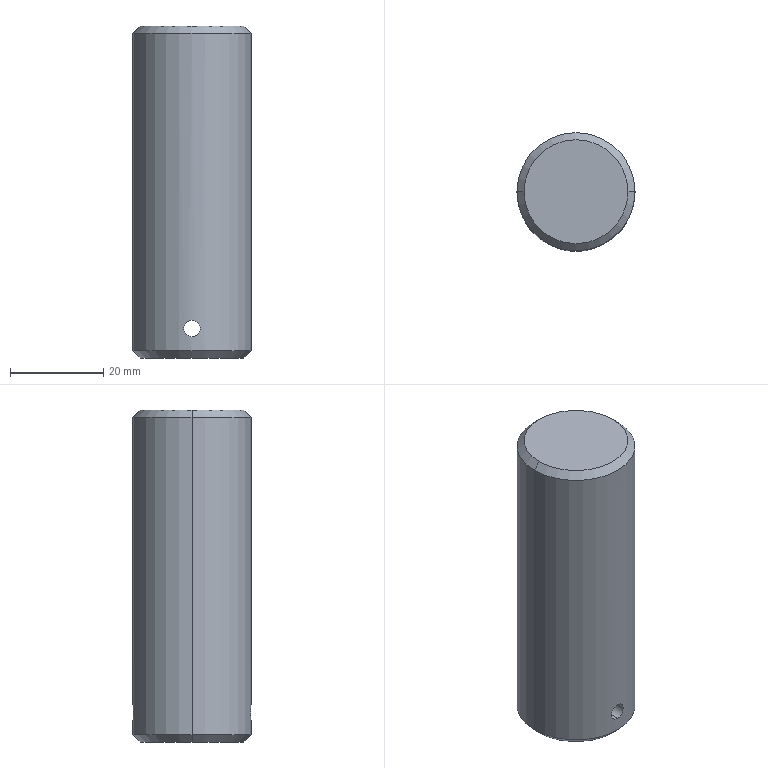Part | SolidWorks | features Chamfer 1, Extrusion 1, ICE 1 | 1 solid | 10 faces | box 25.4 x 25.4 x 71.37 mm | volume 35732 mm3 | cylinder 4 | cone 4 | plane 2 | commonest cylinder face diameters 3.57 x2 25.4 x2
STEP:
#1=CARTESIAN_POINT('',(0.,-12.7,4.565));
#2=VERTEX_POINT('',#1);
#3=CARTESIAN_POINT('',(0.,-12.7,8.135));
#4=VERTEX_POINT('',#3);
#5=CARTESIAN_POINT('',(0.,-12.7,4.565));
#6=CARTESIAN_POINT('',(-0.2331,-12.7,4.565));
#7=CARTESIAN_POINT('',(-0.4682,-12.693,4.612));
#8=CARTESIAN_POINT('',(-0.8979,-12.67,4.79));
#9=CARTESIAN_POINT('',(-1.097,-12.654,4.923));
#10=CARTESIAN_POINT('',(-1.344,-12.629,5.169));
#11=CARTESIAN_POINT('',(-1.419,-12.621,5.261));
#12=CARTESIAN_POINT('',(-1.549,-12.605,5.455));
#13=CARTESIAN_POINT('',(-1.603,-12.598,5.557));
#14=CARTESIAN_POINT('',(-1.693,-12.587,5.773));
#15=CARTESIAN_POINT('',(-1.728,-12.582,5.886));
#16=CARTESIAN_POINT('',(-1.773,-12.576,6.115));
#17=CARTESIAN_POINT('',(-1.785,-12.574,6.231));
#18=CARTESIAN_POINT('',(-1.785,-12.574,6.467));
#19=CARTESIAN_POINT('',(-1.774,-12.576,6.583));
#20=CARTESIAN_POINT('',(-1.728,-12.582,6.811));
#21=CARTESIAN_POINT('',(-1.694,-12.587,6.925));
#22=CARTESIAN_POINT('',(-1.605,-12.598,7.141));
#23=CARTESIAN_POINT('',(-1.55,-12.605,7.243));
#24=CARTESIAN_POINT('',(-1.42,-12.62,7.437));
#25=CARTESIAN_POINT('',(-1.345,-12.629,7.529));
#26=CARTESIAN_POINT('',(-1.099,-12.653,7.776));
#27=CARTESIAN_POINT('',(-0.9,-12.67,7.909));
#28=CARTESIAN_POINT('',(-0.4707,-12.693,8.087));
#29=CARTESIAN_POINT('',(-0.2361,-12.7,8.135));
#30=CARTESIAN_POINT('',(0.,-12.7,8.135));
#31=B_SPLINE_CURVE_WITH_KNOTS('',3,(#5,#6,#7,#8,#9,#10,#11,#12,#13,#14,#15,#16,#17,#18,#19,#20,#21,#22,#23,#24,#25,#26,#27,#28,#29,#30),.UNSPECIFIED.,.F.,.F.,(4,2,2,2,2,2,2,2,2,2,2,2,4),(0.005588,0.006286,0.006984,0.007333,0.007682,0.008032,0.008381,0.00873,0.009079,0.009428,0.009777,0.01048,0.01117),.UNSPECIFIED.);
#32=EDGE_CURVE('',#2,#4,#31,.T.);
#33=ORIENTED_EDGE('',*,*,#32,.F.);
#34=CARTESIAN_POINT('',(0.,12.7,4.565));
#35=VERTEX_POINT('',#34);
#36=CARTESIAN_POINT('',(0.,-12.7,4.565));
#37=DIRECTION('',(0.,1.,0.));
#38=VECTOR('',#37,1000.);
#39=LINE('',#36,#38);
#40=EDGE_CURVE('',#2,#35,#39,.T.);
#41=ORIENTED_EDGE('',*,*,#40,.T.);
#42=CARTESIAN_POINT('',(0.,12.7,8.135));
#43=VERTEX_POINT('',#42);
#44=CARTESIAN_POINT('',(0.,12.7,8.135));
#45=CARTESIAN_POINT('',(-0.1181,12.7,8.135));
#46=CARTESIAN_POINT('',(-0.2342,12.698,8.123));
#47=CARTESIAN_POINT('',(-0.4625,12.692,8.078));
#48=CARTESIAN_POINT('',(-0.576,12.687,8.044));
#49=CARTESIAN_POINT('',(-0.7921,12.676,7.954));
#50=CARTESIAN_POINT('',(-0.8946,12.669,7.899));
#51=CARTESIAN_POINT('',(-1.089,12.654,7.769));
#52=CARTESIAN_POINT('',(-1.18,12.645,7.694));
#53=CARTESIAN_POINT('',(-1.427,12.621,7.447));
#54=CARTESIAN_POINT('',(-1.56,12.604,7.248));
#55=CARTESIAN_POINT('',(-1.738,12.581,6.819));
#56=CARTESIAN_POINT('',(-1.785,12.574,6.584));
#57=CARTESIAN_POINT('',(-1.785,12.574,6.234));
#58=CARTESIAN_POINT('',(-1.773,12.576,6.116));
#59=CARTESIAN_POINT('',(-1.728,12.582,5.887));
#60=CARTESIAN_POINT('',(-1.694,12.587,5.775));
#61=CARTESIAN_POINT('',(-1.604,12.598,5.559));
#62=CARTESIAN_POINT('',(-1.549,12.605,5.455));
#63=CARTESIAN_POINT('',(-1.419,12.621,5.261));
#64=CARTESIAN_POINT('',(-1.345,12.629,5.171));
#65=CARTESIAN_POINT('',(-1.179,12.645,5.005));
#66=CARTESIAN_POINT('',(-1.089,12.654,4.931));
#67=CARTESIAN_POINT('',(-0.8958,12.669,4.802));
#68=CARTESIAN_POINT('',(-0.7914,12.676,4.746));
#69=CARTESIAN_POINT('',(-0.5753,12.687,4.656));
#70=CARTESIAN_POINT('',(-0.4641,12.692,4.622));
#71=CARTESIAN_POINT('',(-0.235,12.698,4.577));
#72=CARTESIAN_POINT('',(-0.1166,12.7,4.565));
#73=CARTESIAN_POINT('',(0.,12.7,4.565));
#74=B_SPLINE_CURVE_WITH_KNOTS('',3,(#44,#45,#46,#47,#48,#49,#50,#51,#52,#53,#54,#55,#56,#57,#58,#59,#60,#61,#62,#63,#64,#65,#66,#67,#68,#69,#70,#71,#72,#73),.UNSPECIFIED.,.F.,.F.,(4,2,2,2,2,2,2,2,2,2,2,2,2,2,4),(0.,0.0003492,0.0006985,0.001048,0.001397,0.002095,0.002794,0.003143,0.003492,0.003842,0.004191,0.00454,0.004889,0.005238,0.005588),.UNSPECIFIED.);
#75=EDGE_CURVE('',#43,#35,#74,.T.);
#76=ORIENTED_EDGE('',*,*,#75,.F.);
#77=CARTESIAN_POINT('',(0.,-12.7,8.135));
#78=DIRECTION('',(0.,1.,0.));
#79=VECTOR('',#78,1000.);
#80=LINE('',#77,#79);
#81=EDGE_CURVE('',#4,#43,#80,.T.);
#82=ORIENTED_EDGE('',*,*,#81,.F.);
#83=EDGE_LOOP('',(#33,#41,#76,#82));
#84=FACE_OUTER_BOUND('',#83,.T.);
#85=CARTESIAN_POINT('',(0.,-12.7,6.35));
#86=DIRECTION('',(0.,1.,0.));
#87=DIRECTION('',(0.,0.,1.));
#88=AXIS2_PLACEMENT_3D('',#85,#86,#87);
#89=CYLINDRICAL_SURFACE('',#88,1.785);
#90=ADVANCED_FACE('',(#84),#89,.F.);
#91=CARTESIAN_POINT('',(11.176,0.,71.37));
#92=VERTEX_POINT('',#91);
#93=CARTESIAN_POINT('',(-11.176,0.,71.37));
#94=VERTEX_POINT('',#93);
#95=CARTESIAN_POINT('',(0.,0.,71.37));
#96=DIRECTION('',(0.,0.,1.));
#97=DIRECTION('',(1.,0.,0.));
#98=AXIS2_PLACEMENT_3D('',#95,#96,#97);
#99=CIRCLE('',#98,11.176);
#100=EDGE_CURVE('',#92,#94,#99,.T.);
#101=ORIENTED_EDGE('',*,*,#100,.F.);
#102=CARTESIAN_POINT('',(12.7,0.,69.846));
#103=VERTEX_POINT('',#102);
#104=CARTESIAN_POINT('',(11.176,0.,71.37));
#105=DIRECTION('',(0.7071,0.,-0.7071));
#106=VECTOR('',#105,1000.);
#107=LINE('',#104,#106);
#108=EDGE_CURVE('',#92,#103,#107,.T.);
#109=ORIENTED_EDGE('',*,*,#108,.T.);
#110=CARTESIAN_POINT('',(-12.7,0.,69.846));
#111=VERTEX_POINT('',#110);
#112=CARTESIAN_POINT('',(0.,0.,69.846));
#113=DIRECTION('',(0.,0.,-1.));
#114=DIRECTION('',(1.,0.,0.));
#115=AXIS2_PLACEMENT_3D('',#112,#113,#114);
#116=CIRCLE('',#115,12.7);
#117=EDGE_CURVE('',#111,#103,#116,.T.);
#118=ORIENTED_EDGE('',*,*,#117,.F.);
#119=CARTESIAN_POINT('',(-11.176,0.,71.37));
#120=DIRECTION('',(-0.7071,0.,-0.7071));
#121=VECTOR('',#120,1000.);
#122=LINE('',#119,#121);
#123=EDGE_CURVE('',#94,#111,#122,.T.);
#124=ORIENTED_EDGE('',*,*,#123,.F.);
#125=EDGE_LOOP('',(#101,#109,#118,#124));
#126=FACE_OUTER_BOUND('',#125,.T.);
#127=CARTESIAN_POINT('',(0.,0.,71.37));
#128=DIRECTION('',(0.,0.,-1.));
#129=DIRECTION('',(-1.,0.,0.));
#130=AXIS2_PLACEMENT_3D('',#127,#128,#129);
#131=CONICAL_SURFACE('',#130,11.176,0.7854);
#132=ADVANCED_FACE('',(#126),#131,.T.);
#133=CARTESIAN_POINT('',(-11.176,0.,0.));
#134=VERTEX_POINT('',#133);
#135=CARTESIAN_POINT('',(11.176,0.,0.));
#136=VERTEX_POINT('',#135);
#137=CARTESIAN_POINT('',(0.,0.,0.));
#138=DIRECTION('',(0.,0.,-1.));
#139=DIRECTION('',(1.,0.,0.));
#140=AXIS2_PLACEMENT_3D('',#137,#138,#139);
#141=CIRCLE('',#140,11.176);
#142=EDGE_CURVE('',#134,#136,#141,.T.);
#143=ORIENTED_EDGE('',*,*,#142,.F.);
#144=CARTESIAN_POINT('',(-12.7,0.,1.524));
#145=VERTEX_POINT('',#144);
#146=CARTESIAN_POINT('',(-12.7,0.,1.524));
#147=DIRECTION('',(-0.7071,0.,0.7071));
#148=VECTOR('',#147,1000.);
#149=LINE('',#146,#148);
#150=EDGE_CURVE('',#134,#145,#149,.T.);
#151=ORIENTED_EDGE('',*,*,#150,.T.);
#152=CARTESIAN_POINT('',(12.7,0.,1.524));
#153=VERTEX_POINT('',#152);
#154=CARTESIAN_POINT('',(0.,0.,1.524));
#155=DIRECTION('',(0.,0.,1.));
#156=DIRECTION('',(1.,0.,0.));
#157=AXIS2_PLACEMENT_3D('',#154,#155,#156);
#158=CIRCLE('',#157,12.7);
#159=EDGE_CURVE('',#153,#145,#158,.T.);
#160=ORIENTED_EDGE('',*,*,#159,.F.);
#161=CARTESIAN_POINT('',(12.7,0.,1.524));
#162=DIRECTION('',(0.7071,0.,0.7071));
#163=VECTOR('',#162,1000.);
#164=LINE('',#161,#163);
#165=EDGE_CURVE('',#136,#153,#164,.T.);
#166=ORIENTED_EDGE('',*,*,#165,.F.);
#167=EDGE_LOOP('',(#143,#151,#160,#166));
#168=FACE_OUTER_BOUND('',#167,.T.);
#169=CARTESIAN_POINT('',(0.,0.,1.524));
#170=DIRECTION('',(0.,0.,1.));
#171=DIRECTION('',(1.,0.,0.));
#172=AXIS2_PLACEMENT_3D('',#169,#170,#171);
#173=CONICAL_SURFACE('',#172,12.7,0.7854);
#174=ADVANCED_FACE('',(#168),#173,.T.);
#175=ORIENTED_EDGE('',*,*,#75,.T.);
#176=CARTESIAN_POINT('',(0.,12.7,4.565));
#177=CARTESIAN_POINT('',(0.2331,12.7,4.565));
#178=CARTESIAN_POINT('',(0.4682,12.693,4.612));
#179=CARTESIAN_POINT('',(0.8979,12.67,4.79));
#180=CARTESIAN_POINT('',(1.097,12.654,4.923));
#181=CARTESIAN_POINT('',(1.344,12.629,5.169));
#182=CARTESIAN_POINT('',(1.419,12.621,5.261));
#183=CARTESIAN_POINT('',(1.549,12.605,5.455));
#184=CARTESIAN_POINT('',(1.603,12.598,5.557));
#185=CARTESIAN_POINT('',(1.693,12.587,5.773));
#186=CARTESIAN_POINT('',(1.728,12.582,5.886));
#187=CARTESIAN_POINT('',(1.773,12.576,6.115));
#188=CARTESIAN_POINT('',(1.785,12.574,6.231));
#189=CARTESIAN_POINT('',(1.785,12.574,6.467));
#190=CARTESIAN_POINT('',(1.774,12.576,6.583));
#191=CARTESIAN_POINT('',(1.728,12.582,6.811));
#192=CARTESIAN_POINT('',(1.694,12.587,6.925));
#193=CARTESIAN_POINT('',(1.605,12.598,7.141));
#194=CARTESIAN_POINT('',(1.55,12.605,7.243));
#195=CARTESIAN_POINT('',(1.42,12.62,7.437));
#196=CARTESIAN_POINT('',(1.345,12.629,7.529));
#197=CARTESIAN_POINT('',(1.099,12.653,7.776));
#198=CARTESIAN_POINT('',(0.9,12.67,7.909));
#199=CARTESIAN_POINT('',(0.4707,12.693,8.087));
#200=CARTESIAN_POINT('',(0.2361,12.7,8.135));
#201=CARTESIAN_POINT('',(0.,12.7,8.135));
#202=B_SPLINE_CURVE_WITH_KNOTS('',3,(#176,#177,#178,#179,#180,#181,#182,#183,#184,#185,#186,#187,#188,#189,#190,#191,#192,#193,#194,#195,#196,#197,#198,#199,#200,#201),.UNSPECIFIED.,.F.,.F.,(4,2,2,2,2,2,2,2,2,2,2,2,4),(0.005588,0.006286,0.006984,0.007333,0.007682,0.008032,0.008381,0.00873,0.009079,0.009428,0.009777,0.01048,0.01117),.UNSPECIFIED.);
#203=EDGE_CURVE('',#35,#43,#202,.T.);
#204=ORIENTED_EDGE('',*,*,#203,.T.);
#205=EDGE_LOOP('',(#175,#204));
#206=FACE_BOUND('',#205,.T.);
#207=ORIENTED_EDGE('',*,*,#117,.T.);
#208=CARTESIAN_POINT('',(12.7,0.,71.37));
#209=DIRECTION('',(0.,0.,-1.));
#210=VECTOR('',#209,1000.);
#211=LINE('',#208,#210);
#212=EDGE_CURVE('',#103,#153,#211,.T.);
#213=ORIENTED_EDGE('',*,*,#212,.T.);
#214=ORIENTED_EDGE('',*,*,#159,.T.);
#215=CARTESIAN_POINT('',(-12.7,0.,71.37));
#216=DIRECTION('',(0.,0.,-1.));
#217=VECTOR('',#216,1000.);
#218=LINE('',#215,#217);
#219=EDGE_CURVE('',#111,#145,#218,.T.);
#220=ORIENTED_EDGE('',*,*,#219,.F.);
#221=EDGE_LOOP('',(#207,#213,#214,#220));
#222=FACE_OUTER_BOUND('',#221,.T.);
#223=CARTESIAN_POINT('',(0.,0.,71.37));
#224=DIRECTION('',(0.,0.,-1.));
#225=DIRECTION('',(-1.,0.,0.));
#226=AXIS2_PLACEMENT_3D('',#223,#224,#225);
#227=CYLINDRICAL_SURFACE('',#226,12.7);
#228=ADVANCED_FACE('',(#206,#222),#227,.T.);
#229=ORIENTED_EDGE('',*,*,#212,.F.);
#230=CARTESIAN_POINT('',(0.,0.,69.846));
#231=DIRECTION('',(0.,0.,-1.));
#232=DIRECTION('',(1.,0.,0.));
#233=AXIS2_PLACEMENT_3D('',#230,#231,#232);
#234=CIRCLE('',#233,12.7);
#235=EDGE_CURVE('',#103,#111,#234,.T.);
#236=ORIENTED_EDGE('',*,*,#235,.T.);
#237=ORIENTED_EDGE('',*,*,#219,.T.);
#238=CARTESIAN_POINT('',(0.,0.,1.524));
#239=DIRECTION('',(0.,0.,1.));
#240=DIRECTION('',(1.,0.,0.));
#241=AXIS2_PLACEMENT_3D('',#238,#239,#240);
#242=CIRCLE('',#241,12.7);
#243=EDGE_CURVE('',#145,#153,#242,.T.);
#244=ORIENTED_EDGE('',*,*,#243,.T.);
#245=EDGE_LOOP('',(#229,#236,#237,#244));
#246=FACE_OUTER_BOUND('',#245,.T.);
#247=CARTESIAN_POINT('',(0.,-12.7,8.135));
#248=CARTESIAN_POINT('',(0.1181,-12.7,8.135));
#249=CARTESIAN_POINT('',(0.2342,-12.698,8.123));
#250=CARTESIAN_POINT('',(0.4625,-12.692,8.078));
#251=CARTESIAN_POINT('',(0.576,-12.687,8.044));
#252=CARTESIAN_POINT('',(0.7921,-12.676,7.954));
#253=CARTESIAN_POINT('',(0.8946,-12.669,7.899));
#254=CARTESIAN_POINT('',(1.089,-12.654,7.769));
#255=CARTESIAN_POINT('',(1.18,-12.645,7.694));
#256=CARTESIAN_POINT('',(1.427,-12.621,7.447));
#257=CARTESIAN_POINT('',(1.56,-12.604,7.248));
#258=CARTESIAN_POINT('',(1.738,-12.581,6.819));
#259=CARTESIAN_POINT('',(1.785,-12.574,6.584));
#260=CARTESIAN_POINT('',(1.785,-12.574,6.234));
#261=CARTESIAN_POINT('',(1.773,-12.576,6.116));
#262=CARTESIAN_POINT('',(1.728,-12.582,5.887));
#263=CARTESIAN_POINT('',(1.694,-12.587,5.775));
#264=CARTESIAN_POINT('',(1.604,-12.598,5.559));
#265=CARTESIAN_POINT('',(1.549,-12.605,5.455));
#266=CARTESIAN_POINT('',(1.419,-12.621,5.261));
#267=CARTESIAN_POINT('',(1.345,-12.629,5.171));
#268=CARTESIAN_POINT('',(1.179,-12.645,5.005));
#269=CARTESIAN_POINT('',(1.089,-12.654,4.931));
#270=CARTESIAN_POINT('',(0.8958,-12.669,4.802));
#271=CARTESIAN_POINT('',(0.7914,-12.676,4.746));
#272=CARTESIAN_POINT('',(0.5753,-12.687,4.656));
#273=CARTESIAN_POINT('',(0.4641,-12.692,4.622));
#274=CARTESIAN_POINT('',(0.235,-12.698,4.577));
#275=CARTESIAN_POINT('',(0.1166,-12.7,4.565));
#276=CARTESIAN_POINT('',(0.,-12.7,4.565));
#277=B_SPLINE_CURVE_WITH_KNOTS('',3,(#247,#248,#249,#250,#251,#252,#253,#254,#255,#256,#257,#258,#259,#260,#261,#262,#263,#264,#265,#266,#267,#268,#269,#270,#271,#272,#273,#274,#275,#276),.UNSPECIFIED.,.F.,.F.,(4,2,2,2,2,2,2,2,2,2,2,2,2,2,4),(0.,0.0003492,0.0006985,0.001048,0.001397,0.002095,0.002794,0.003143,0.003492,0.003842,0.004191,0.00454,0.004889,0.005238,0.005588),.UNSPECIFIED.);
#278=EDGE_CURVE('',#4,#2,#277,.T.);
#279=ORIENTED_EDGE('',*,*,#278,.T.);
#280=ORIENTED_EDGE('',*,*,#32,.T.);
#281=EDGE_LOOP('',(#279,#280));
#282=FACE_BOUND('',#281,.T.);
#283=CARTESIAN_POINT('',(0.,0.,71.37));
#284=DIRECTION('',(0.,0.,-1.));
#285=DIRECTION('',(-1.,0.,0.));
#286=AXIS2_PLACEMENT_3D('',#283,#284,#285);
#287=CYLINDRICAL_SURFACE('',#286,12.7);
#288=ADVANCED_FACE('',(#246,#282),#287,.T.);
#289=CARTESIAN_POINT('',(0.,0.,71.37));
#290=DIRECTION('',(0.,0.,1.));
#291=DIRECTION('',(1.,0.,0.));
#292=AXIS2_PLACEMENT_3D('',#289,#290,#291);
#293=CIRCLE('',#292,11.176);
#294=EDGE_CURVE('',#94,#92,#293,.T.);
#295=ORIENTED_EDGE('',*,*,#294,.T.);
#296=ORIENTED_EDGE('',*,*,#100,.T.);
#297=EDGE_LOOP('',(#295,#296));
#298=FACE_OUTER_BOUND('',#297,.T.);
#299=CARTESIAN_POINT('',(0.,0.,71.37));
#300=DIRECTION('',(0.,0.,1.));
#301=DIRECTION('',(1.,0.,0.));
#302=AXIS2_PLACEMENT_3D('',#299,#300,#301);
#303=PLANE('',#302);
#304=ADVANCED_FACE('',(#298),#303,.T.);
#305=CARTESIAN_POINT('',(0.,0.,0.));
#306=DIRECTION('',(0.,0.,-1.));
#307=DIRECTION('',(1.,0.,0.));
#308=AXIS2_PLACEMENT_3D('',#305,#306,#307);
#309=CIRCLE('',#308,11.176);
#310=EDGE_CURVE('',#136,#134,#309,.T.);
#311=ORIENTED_EDGE('',*,*,#310,.T.);
#312=ORIENTED_EDGE('',*,*,#142,.T.);
#313=EDGE_LOOP('',(#311,#312));
#314=FACE_OUTER_BOUND('',#313,.T.);
#315=CARTESIAN_POINT('',(0.,0.,0.));
#316=DIRECTION('',(0.,0.,1.));
#317=DIRECTION('',(1.,0.,0.));
#318=AXIS2_PLACEMENT_3D('',#315,#316,#317);
#319=PLANE('',#318);
#320=ADVANCED_FACE('',(#314),#319,.F.);
#321=ORIENTED_EDGE('',*,*,#150,.F.);
#322=ORIENTED_EDGE('',*,*,#310,.F.);
#323=ORIENTED_EDGE('',*,*,#165,.T.);
#324=ORIENTED_EDGE('',*,*,#243,.F.);
#325=EDGE_LOOP('',(#321,#322,#323,#324));
#326=FACE_OUTER_BOUND('',#325,.T.);
#327=CARTESIAN_POINT('',(0.,0.,1.524));
#328=DIRECTION('',(0.,0.,1.));
#329=DIRECTION('',(1.,0.,0.));
#330=AXIS2_PLACEMENT_3D('',#327,#328,#329);
#331=CONICAL_SURFACE('',#330,12.7,0.7854);
#332=ADVANCED_FACE('',(#326),#331,.T.);
#333=ORIENTED_EDGE('',*,*,#108,.F.);
#334=ORIENTED_EDGE('',*,*,#294,.F.);
#335=ORIENTED_EDGE('',*,*,#123,.T.);
#336=ORIENTED_EDGE('',*,*,#235,.F.);
#337=EDGE_LOOP('',(#333,#334,#335,#336));
#338=FACE_OUTER_BOUND('',#337,.T.);
#339=CARTESIAN_POINT('',(0.,0.,71.37));
#340=DIRECTION('',(0.,0.,-1.));
#341=DIRECTION('',(-1.,0.,0.));
#342=AXIS2_PLACEMENT_3D('',#339,#340,#341);
#343=CONICAL_SURFACE('',#342,11.176,0.7854);
#344=ADVANCED_FACE('',(#338),#343,.T.);
#345=ORIENTED_EDGE('',*,*,#40,.F.);
#346=ORIENTED_EDGE('',*,*,#278,.F.);
#347=ORIENTED_EDGE('',*,*,#81,.T.);
#348=ORIENTED_EDGE('',*,*,#203,.F.);
#349=EDGE_LOOP('',(#345,#346,#347,#348));
#350=FACE_OUTER_BOUND('',#349,.T.);
#351=CARTESIAN_POINT('',(0.,-12.7,6.35));
#352=DIRECTION('',(0.,1.,0.));
#353=DIRECTION('',(0.,0.,1.));
#354=AXIS2_PLACEMENT_3D('',#351,#352,#353);
#355=CYLINDRICAL_SURFACE('',#354,1.785);
#356=ADVANCED_FACE('',(#350),#355,.F.);
#357=CLOSED_SHELL('',(#90,#132,#174,#228,#288,#304,#320,#332,#344,#356));
#358=MANIFOLD_SOLID_BREP('',#357);
#359=CARTESIAN_POINT('',(0.,0.,0.));
#360=DIRECTION('',(0.,0.,1.));
#361=DIRECTION('',(1.,0.,0.));
#362=AXIS2_PLACEMENT_3D('',#359,#360,#361);
#363=(LENGTH_UNIT()NAMED_UNIT(*)SI_UNIT(.MILLI.,.METRE.));
#364=UNCERTAINTY_MEASURE_WITH_UNIT(LENGTH_MEASURE(0.00001),#363,'','');
#365=(NAMED_UNIT(*)PLANE_ANGLE_UNIT()SI_UNIT($,.RADIAN.));
#366=(NAMED_UNIT(*)SI_UNIT($,.STERADIAN.)SOLID_ANGLE_UNIT());
#367=(GEOMETRIC_REPRESENTATION_CONTEXT(3)GLOBAL_UNCERTAINTY_ASSIGNED_CONTEXT((#364))GLOBAL_UNIT_ASSIGNED_CONTEXT((#363,#365,#366))REPRESENTATION_CONTEXT('',''));
#368=ADVANCED_BREP_SHAPE_REPRESENTATION('',(#358,#362),#367);